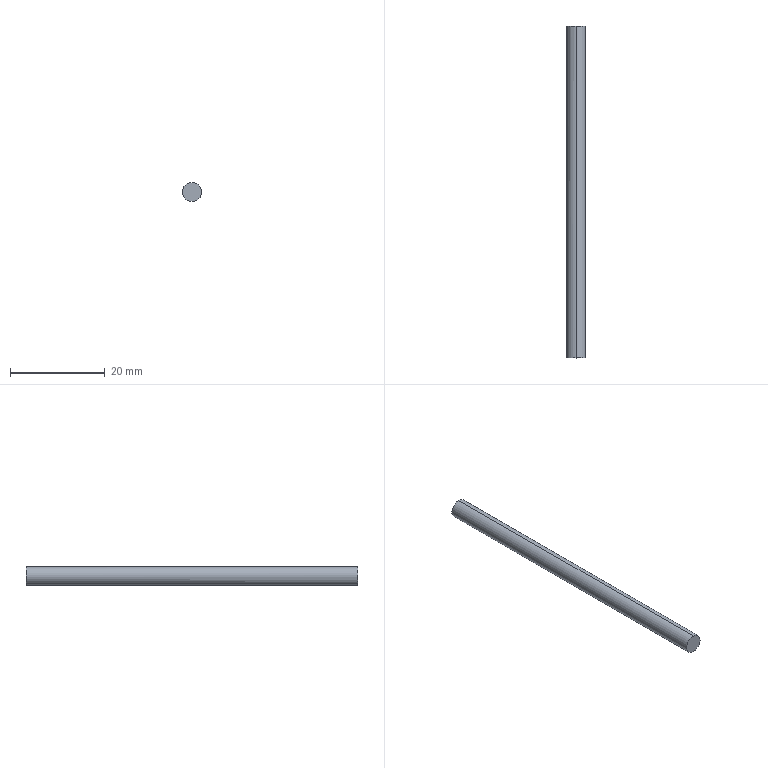Part | SolidWorks | features BaseBody 1 | 1 solid | 4 faces | box 4 x 70 x 4 mm | volume 879.661 mm3 | cylinder 2 | plane 2 | commonest cylinder face diameters 4 x2
STEP:
#1=CARTESIAN_POINT('',(0.,70.,2.));
#2=VERTEX_POINT('',#1);
#3=CARTESIAN_POINT('',(0.,70.,-2.));
#4=VERTEX_POINT('',#3);
#5=CARTESIAN_POINT('',(0.,70.,2.));
#6=CARTESIAN_POINT('',(0.2652,70.,2.));
#7=CARTESIAN_POINT('',(0.5203,70.,1.949));
#8=CARTESIAN_POINT('',(1.01,70.,1.746));
#9=CARTESIAN_POINT('',(1.227,70.,1.602));
#10=CARTESIAN_POINT('',(1.602,70.,1.227));
#11=CARTESIAN_POINT('',(1.746,70.,1.01));
#12=CARTESIAN_POINT('',(1.949,70.,0.5203));
#13=CARTESIAN_POINT('',(2.,70.,0.2652));
#14=CARTESIAN_POINT('',(2.,70.,-0.2652));
#15=CARTESIAN_POINT('',(1.949,70.,-0.5203));
#16=CARTESIAN_POINT('',(1.746,70.,-1.01));
#17=CARTESIAN_POINT('',(1.602,70.,-1.227));
#18=CARTESIAN_POINT('',(1.227,70.,-1.602));
#19=CARTESIAN_POINT('',(1.01,70.,-1.746));
#20=CARTESIAN_POINT('',(0.5203,70.,-1.949));
#21=CARTESIAN_POINT('',(0.2652,70.,-2.));
#22=CARTESIAN_POINT('',(0.,70.,-2.));
#23=B_SPLINE_CURVE_WITH_KNOTS('',3,(#5,#6,#7,#8,#9,#10,#11,#12,#13,#14,#15,#16,#17,#18,#19,#20,#21,#22),.UNSPECIFIED.,.F.,.F.,(4,2,2,2,2,2,2,2,4),(4.712,5.105,5.498,5.89,6.283,6.676,7.069,7.461,7.854),.UNSPECIFIED.);
#24=EDGE_CURVE('',#2,#4,#23,.T.);
#25=ORIENTED_EDGE('',*,*,#24,.F.);
#26=CARTESIAN_POINT('',(0.,0.,2.));
#27=VERTEX_POINT('',#26);
#28=CARTESIAN_POINT('',(0.,70.,2.));
#29=DIRECTION('',(0.,-1.,0.));
#30=VECTOR('',#29,1000.);
#31=LINE('',#28,#30);
#32=EDGE_CURVE('',#2,#27,#31,.T.);
#33=ORIENTED_EDGE('',*,*,#32,.T.);
#34=CARTESIAN_POINT('',(0.,0.,-2.));
#35=VERTEX_POINT('',#34);
#36=CARTESIAN_POINT('',(0.,0.,2.));
#37=CARTESIAN_POINT('',(0.2618,0.,2.));
#38=CARTESIAN_POINT('',(0.5235,0.,1.948));
#39=CARTESIAN_POINT('',(1.007,0.,1.748));
#40=CARTESIAN_POINT('',(1.229,0.,1.599));
#41=CARTESIAN_POINT('',(1.599,0.,1.229));
#42=CARTESIAN_POINT('',(1.748,0.,1.007));
#43=CARTESIAN_POINT('',(1.948,0.,0.5235));
#44=CARTESIAN_POINT('',(2.,0.,0.2618));
#45=CARTESIAN_POINT('',(2.,0.,-0.2618));
#46=CARTESIAN_POINT('',(1.948,0.,-0.5235));
#47=CARTESIAN_POINT('',(1.748,0.,-1.007));
#48=CARTESIAN_POINT('',(1.599,0.,-1.229));
#49=CARTESIAN_POINT('',(1.229,0.,-1.599));
#50=CARTESIAN_POINT('',(1.007,0.,-1.748));
#51=CARTESIAN_POINT('',(0.5235,0.,-1.948));
#52=CARTESIAN_POINT('',(0.2618,0.,-2.));
#53=CARTESIAN_POINT('',(0.,0.,-2.));
#54=B_SPLINE_CURVE_WITH_KNOTS('',3,(#36,#37,#38,#39,#40,#41,#42,#43,#44,#45,#46,#47,#48,#49,#50,#51,#52,#53),.UNSPECIFIED.,.F.,.F.,(4,2,2,2,2,2,2,2,4),(4.712,5.105,5.498,5.89,6.283,6.676,7.069,7.461,7.854),.UNSPECIFIED.);
#55=EDGE_CURVE('',#27,#35,#54,.T.);
#56=ORIENTED_EDGE('',*,*,#55,.T.);
#57=CARTESIAN_POINT('',(0.,70.,-2.));
#58=DIRECTION('',(0.,-1.,0.));
#59=VECTOR('',#58,1000.);
#60=LINE('',#57,#59);
#61=EDGE_CURVE('',#4,#35,#60,.T.);
#62=ORIENTED_EDGE('',*,*,#61,.F.);
#63=EDGE_LOOP('',(#25,#33,#56,#62));
#64=FACE_OUTER_BOUND('',#63,.T.);
#65=CARTESIAN_POINT('',(0.,70.,0.));
#66=DIRECTION('',(0.,-1.,0.));
#67=DIRECTION('',(0.,0.,-1.));
#68=AXIS2_PLACEMENT_3D('',#65,#66,#67);
#69=CYLINDRICAL_SURFACE('',#68,2.);
#70=ADVANCED_FACE('',(#64),#69,.T.);
#71=ORIENTED_EDGE('',*,*,#32,.F.);
#72=CARTESIAN_POINT('',(0.,70.,-2.));
#73=CARTESIAN_POINT('',(-0.2652,70.,-2.));
#74=CARTESIAN_POINT('',(-0.5203,70.,-1.949));
#75=CARTESIAN_POINT('',(-1.01,70.,-1.746));
#76=CARTESIAN_POINT('',(-1.227,70.,-1.602));
#77=CARTESIAN_POINT('',(-1.602,70.,-1.227));
#78=CARTESIAN_POINT('',(-1.746,70.,-1.01));
#79=CARTESIAN_POINT('',(-1.949,70.,-0.5203));
#80=CARTESIAN_POINT('',(-2.,70.,-0.2652));
#81=CARTESIAN_POINT('',(-2.,70.,0.2652));
#82=CARTESIAN_POINT('',(-1.949,70.,0.5203));
#83=CARTESIAN_POINT('',(-1.746,70.,1.01));
#84=CARTESIAN_POINT('',(-1.602,70.,1.227));
#85=CARTESIAN_POINT('',(-1.227,70.,1.602));
#86=CARTESIAN_POINT('',(-1.01,70.,1.746));
#87=CARTESIAN_POINT('',(-0.5203,70.,1.949));
#88=CARTESIAN_POINT('',(-0.2652,70.,2.));
#89=CARTESIAN_POINT('',(0.,70.,2.));
#90=B_SPLINE_CURVE_WITH_KNOTS('',3,(#72,#73,#74,#75,#76,#77,#78,#79,#80,#81,#82,#83,#84,#85,#86,#87,#88,#89),.UNSPECIFIED.,.F.,.F.,(4,2,2,2,2,2,2,2,4),(1.571,1.963,2.356,2.749,3.142,3.534,3.927,4.32,4.712),.UNSPECIFIED.);
#91=EDGE_CURVE('',#4,#2,#90,.T.);
#92=ORIENTED_EDGE('',*,*,#91,.F.);
#93=ORIENTED_EDGE('',*,*,#61,.T.);
#94=CARTESIAN_POINT('',(0.,0.,-2.));
#95=CARTESIAN_POINT('',(-0.2618,0.,-2.));
#96=CARTESIAN_POINT('',(-0.5235,0.,-1.948));
#97=CARTESIAN_POINT('',(-1.007,0.,-1.748));
#98=CARTESIAN_POINT('',(-1.229,0.,-1.599));
#99=CARTESIAN_POINT('',(-1.599,0.,-1.229));
#100=CARTESIAN_POINT('',(-1.748,0.,-1.007));
#101=CARTESIAN_POINT('',(-1.948,0.,-0.5235));
#102=CARTESIAN_POINT('',(-2.,0.,-0.2618));
#103=CARTESIAN_POINT('',(-2.,0.,0.2618));
#104=CARTESIAN_POINT('',(-1.948,0.,0.5235));
#105=CARTESIAN_POINT('',(-1.748,0.,1.007));
#106=CARTESIAN_POINT('',(-1.599,0.,1.229));
#107=CARTESIAN_POINT('',(-1.229,0.,1.599));
#108=CARTESIAN_POINT('',(-1.007,0.,1.748));
#109=CARTESIAN_POINT('',(-0.5235,0.,1.948));
#110=CARTESIAN_POINT('',(-0.2618,0.,2.));
#111=CARTESIAN_POINT('',(0.,0.,2.));
#112=B_SPLINE_CURVE_WITH_KNOTS('',3,(#94,#95,#96,#97,#98,#99,#100,#101,#102,#103,#104,#105,#106,#107,#108,#109,#110,#111),.UNSPECIFIED.,.F.,.F.,(4,2,2,2,2,2,2,2,4),(1.571,1.963,2.356,2.749,3.142,3.534,3.927,4.32,4.712),.UNSPECIFIED.);
#113=EDGE_CURVE('',#35,#27,#112,.T.);
#114=ORIENTED_EDGE('',*,*,#113,.T.);
#115=EDGE_LOOP('',(#71,#92,#93,#114));
#116=FACE_OUTER_BOUND('',#115,.T.);
#117=CARTESIAN_POINT('',(0.,70.,0.));
#118=DIRECTION('',(0.,-1.,0.));
#119=DIRECTION('',(0.,0.,-1.));
#120=AXIS2_PLACEMENT_3D('',#117,#118,#119);
#121=CYLINDRICAL_SURFACE('',#120,2.);
#122=ADVANCED_FACE('',(#116),#121,.T.);
#123=ORIENTED_EDGE('',*,*,#91,.T.);
#124=ORIENTED_EDGE('',*,*,#24,.T.);
#125=EDGE_LOOP('',(#123,#124));
#126=FACE_OUTER_BOUND('',#125,.T.);
#127=CARTESIAN_POINT('',(0.,70.,0.));
#128=DIRECTION('',(0.,1.,0.));
#129=DIRECTION('',(0.,0.,1.));
#130=AXIS2_PLACEMENT_3D('',#127,#128,#129);
#131=PLANE('',#130);
#132=ADVANCED_FACE('',(#126),#131,.T.);
#133=ORIENTED_EDGE('',*,*,#113,.F.);
#134=ORIENTED_EDGE('',*,*,#55,.F.);
#135=EDGE_LOOP('',(#133,#134));
#136=FACE_OUTER_BOUND('',#135,.T.);
#137=CARTESIAN_POINT('',(0.,0.,0.));
#138=DIRECTION('',(0.,1.,0.));
#139=DIRECTION('',(0.,0.,1.));
#140=AXIS2_PLACEMENT_3D('',#137,#138,#139);
#141=PLANE('',#140);
#142=ADVANCED_FACE('',(#136),#141,.F.);
#143=CLOSED_SHELL('',(#70,#122,#132,#142));
#144=MANIFOLD_SOLID_BREP('',#143);
#145=CARTESIAN_POINT('',(0.,0.,0.));
#146=DIRECTION('',(0.,0.,1.));
#147=DIRECTION('',(1.,0.,0.));
#148=AXIS2_PLACEMENT_3D('',#145,#146,#147);
#149=(LENGTH_UNIT()NAMED_UNIT(*)SI_UNIT(.MILLI.,.METRE.));
#150=UNCERTAINTY_MEASURE_WITH_UNIT(LENGTH_MEASURE(0.00001),#149,'','');
#151=(NAMED_UNIT(*)PLANE_ANGLE_UNIT()SI_UNIT($,.RADIAN.));
#152=(NAMED_UNIT(*)SI_UNIT($,.STERADIAN.)SOLID_ANGLE_UNIT());
#153=(GEOMETRIC_REPRESENTATION_CONTEXT(3)GLOBAL_UNCERTAINTY_ASSIGNED_CONTEXT((#150))GLOBAL_UNIT_ASSIGNED_CONTEXT((#149,#151,#152))REPRESENTATION_CONTEXT('',''));
#154=ADVANCED_BREP_SHAPE_REPRESENTATION('',(#144,#148),#153);